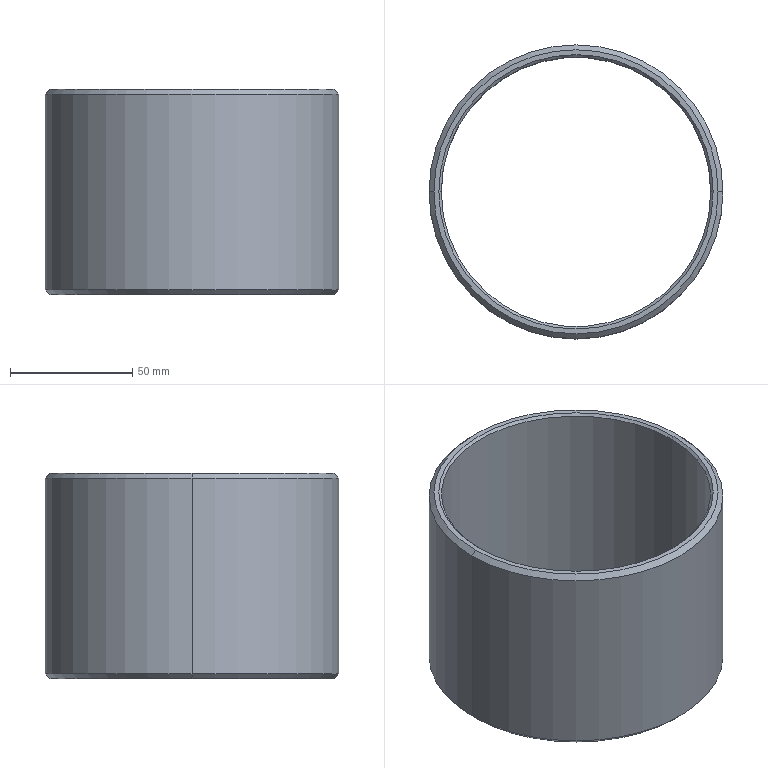Part | SolidWorks | features Chamfer 2, Extrusion 1 | 1 solid | 14 faces | box 120 x 120 x 84 mm | volume 149900 mm3 | cone 8 | cylinder 4 | plane 2 | commonest cylinder face diameters 110 x2 120 x2
STEP:
#1=CARTESIAN_POINT('',(-55.,0.,41.));
#2=VERTEX_POINT('',#1);
#3=CARTESIAN_POINT('',(55.,0.,41.));
#4=VERTEX_POINT('',#3);
#5=CARTESIAN_POINT('',(0.,0.,41.));
#6=DIRECTION('',(0.,0.,1.));
#7=DIRECTION('',(1.,0.,0.));
#8=AXIS2_PLACEMENT_3D('',#5,#6,#7);
#9=CIRCLE('',#8,55.);
#10=EDGE_CURVE('',#2,#4,#9,.T.);
#11=ORIENTED_EDGE('',*,*,#10,.F.);
#12=CARTESIAN_POINT('',(-56.,0.,42.));
#13=VERTEX_POINT('',#12);
#14=CARTESIAN_POINT('',(-55.,0.,41.));
#15=DIRECTION('',(-0.7071,0.,0.7071));
#16=VECTOR('',#15,1000.);
#17=LINE('',#14,#16);
#18=EDGE_CURVE('',#2,#13,#17,.T.);
#19=ORIENTED_EDGE('',*,*,#18,.T.);
#20=CARTESIAN_POINT('',(56.,0.,42.));
#21=VERTEX_POINT('',#20);
#22=CARTESIAN_POINT('',(0.,0.,42.));
#23=DIRECTION('',(0.,0.,-1.));
#24=DIRECTION('',(1.,0.,0.));
#25=AXIS2_PLACEMENT_3D('',#22,#23,#24);
#26=CIRCLE('',#25,56.);
#27=EDGE_CURVE('',#21,#13,#26,.T.);
#28=ORIENTED_EDGE('',*,*,#27,.F.);
#29=CARTESIAN_POINT('',(55.,0.,41.));
#30=DIRECTION('',(0.7071,0.,0.7071));
#31=VECTOR('',#30,1000.);
#32=LINE('',#29,#31);
#33=EDGE_CURVE('',#4,#21,#32,.T.);
#34=ORIENTED_EDGE('',*,*,#33,.F.);
#35=EDGE_LOOP('',(#11,#19,#28,#34));
#36=FACE_OUTER_BOUND('',#35,.T.);
#37=CARTESIAN_POINT('',(0.,0.,41.));
#38=DIRECTION('',(0.,0.,1.));
#39=DIRECTION('',(1.,0.,0.));
#40=AXIS2_PLACEMENT_3D('',#37,#38,#39);
#41=CONICAL_SURFACE('',#40,55.,0.7854);
#42=ADVANCED_FACE('',(#36),#41,.F.);
#43=CARTESIAN_POINT('',(55.,0.,-41.));
#44=VERTEX_POINT('',#43);
#45=CARTESIAN_POINT('',(-55.,0.,-41.));
#46=VERTEX_POINT('',#45);
#47=CARTESIAN_POINT('',(0.,0.,-41.));
#48=DIRECTION('',(0.,0.,-1.));
#49=DIRECTION('',(1.,0.,0.));
#50=AXIS2_PLACEMENT_3D('',#47,#48,#49);
#51=CIRCLE('',#50,55.);
#52=EDGE_CURVE('',#44,#46,#51,.T.);
#53=ORIENTED_EDGE('',*,*,#52,.F.);
#54=CARTESIAN_POINT('',(56.,0.,-42.));
#55=VERTEX_POINT('',#54);
#56=CARTESIAN_POINT('',(56.,0.,-42.));
#57=DIRECTION('',(0.7071,0.,-0.7071));
#58=VECTOR('',#57,1000.);
#59=LINE('',#56,#58);
#60=EDGE_CURVE('',#44,#55,#59,.T.);
#61=ORIENTED_EDGE('',*,*,#60,.T.);
#62=CARTESIAN_POINT('',(-56.,0.,-42.));
#63=VERTEX_POINT('',#62);
#64=CARTESIAN_POINT('',(0.,0.,-42.));
#65=DIRECTION('',(0.,0.,1.));
#66=DIRECTION('',(1.,0.,0.));
#67=AXIS2_PLACEMENT_3D('',#64,#65,#66);
#68=CIRCLE('',#67,56.);
#69=EDGE_CURVE('',#63,#55,#68,.T.);
#70=ORIENTED_EDGE('',*,*,#69,.F.);
#71=CARTESIAN_POINT('',(-56.,0.,-42.));
#72=DIRECTION('',(-0.7071,0.,-0.7071));
#73=VECTOR('',#72,1000.);
#74=LINE('',#71,#73);
#75=EDGE_CURVE('',#46,#63,#74,.T.);
#76=ORIENTED_EDGE('',*,*,#75,.F.);
#77=EDGE_LOOP('',(#53,#61,#70,#76));
#78=FACE_OUTER_BOUND('',#77,.T.);
#79=CARTESIAN_POINT('',(0.,0.,-42.));
#80=DIRECTION('',(0.,0.,-1.));
#81=DIRECTION('',(-1.,0.,0.));
#82=AXIS2_PLACEMENT_3D('',#79,#80,#81);
#83=CONICAL_SURFACE('',#82,56.,0.7854);
#84=ADVANCED_FACE('',(#78),#83,.F.);
#85=CARTESIAN_POINT('',(-58.,0.,-42.));
#86=VERTEX_POINT('',#85);
#87=CARTESIAN_POINT('',(58.,0.,-42.));
#88=VERTEX_POINT('',#87);
#89=CARTESIAN_POINT('',(0.,0.,-42.));
#90=DIRECTION('',(0.,0.,-1.));
#91=DIRECTION('',(1.,0.,0.));
#92=AXIS2_PLACEMENT_3D('',#89,#90,#91);
#93=CIRCLE('',#92,58.);
#94=EDGE_CURVE('',#86,#88,#93,.T.);
#95=ORIENTED_EDGE('',*,*,#94,.F.);
#96=CARTESIAN_POINT('',(-60.,0.,-40.));
#97=VERTEX_POINT('',#96);
#98=CARTESIAN_POINT('',(-60.,0.,-40.));
#99=DIRECTION('',(-0.7071,0.,0.7071));
#100=VECTOR('',#99,1000.);
#101=LINE('',#98,#100);
#102=EDGE_CURVE('',#86,#97,#101,.T.);
#103=ORIENTED_EDGE('',*,*,#102,.T.);
#104=CARTESIAN_POINT('',(60.,0.,-40.));
#105=VERTEX_POINT('',#104);
#106=CARTESIAN_POINT('',(0.,0.,-40.));
#107=DIRECTION('',(0.,0.,1.));
#108=DIRECTION('',(1.,0.,0.));
#109=AXIS2_PLACEMENT_3D('',#106,#107,#108);
#110=CIRCLE('',#109,60.);
#111=EDGE_CURVE('',#105,#97,#110,.T.);
#112=ORIENTED_EDGE('',*,*,#111,.F.);
#113=CARTESIAN_POINT('',(60.,0.,-40.));
#114=DIRECTION('',(0.7071,0.,0.7071));
#115=VECTOR('',#114,1000.);
#116=LINE('',#113,#115);
#117=EDGE_CURVE('',#88,#105,#116,.T.);
#118=ORIENTED_EDGE('',*,*,#117,.F.);
#119=EDGE_LOOP('',(#95,#103,#112,#118));
#120=FACE_OUTER_BOUND('',#119,.T.);
#121=CARTESIAN_POINT('',(0.,0.,-40.));
#122=DIRECTION('',(0.,0.,1.));
#123=DIRECTION('',(1.,0.,0.));
#124=AXIS2_PLACEMENT_3D('',#121,#122,#123);
#125=CONICAL_SURFACE('',#124,60.,0.7854);
#126=ADVANCED_FACE('',(#120),#125,.T.);
#127=CARTESIAN_POINT('',(58.,0.,42.));
#128=VERTEX_POINT('',#127);
#129=CARTESIAN_POINT('',(-58.,0.,42.));
#130=VERTEX_POINT('',#129);
#131=CARTESIAN_POINT('',(0.,0.,42.));
#132=DIRECTION('',(0.,0.,1.));
#133=DIRECTION('',(1.,0.,0.));
#134=AXIS2_PLACEMENT_3D('',#131,#132,#133);
#135=CIRCLE('',#134,58.);
#136=EDGE_CURVE('',#128,#130,#135,.T.);
#137=ORIENTED_EDGE('',*,*,#136,.F.);
#138=CARTESIAN_POINT('',(60.,0.,40.));
#139=VERTEX_POINT('',#138);
#140=CARTESIAN_POINT('',(58.,0.,42.));
#141=DIRECTION('',(0.7071,0.,-0.7071));
#142=VECTOR('',#141,1000.);
#143=LINE('',#140,#142);
#144=EDGE_CURVE('',#128,#139,#143,.T.);
#145=ORIENTED_EDGE('',*,*,#144,.T.);
#146=CARTESIAN_POINT('',(-60.,0.,40.));
#147=VERTEX_POINT('',#146);
#148=CARTESIAN_POINT('',(0.,0.,40.));
#149=DIRECTION('',(0.,0.,-1.));
#150=DIRECTION('',(1.,0.,0.));
#151=AXIS2_PLACEMENT_3D('',#148,#149,#150);
#152=CIRCLE('',#151,60.);
#153=EDGE_CURVE('',#147,#139,#152,.T.);
#154=ORIENTED_EDGE('',*,*,#153,.F.);
#155=CARTESIAN_POINT('',(-58.,0.,42.));
#156=DIRECTION('',(-0.7071,0.,-0.7071));
#157=VECTOR('',#156,1000.);
#158=LINE('',#155,#157);
#159=EDGE_CURVE('',#130,#147,#158,.T.);
#160=ORIENTED_EDGE('',*,*,#159,.F.);
#161=EDGE_LOOP('',(#137,#145,#154,#160));
#162=FACE_OUTER_BOUND('',#161,.T.);
#163=CARTESIAN_POINT('',(0.,0.,42.));
#164=DIRECTION('',(0.,0.,-1.));
#165=DIRECTION('',(-1.,0.,0.));
#166=AXIS2_PLACEMENT_3D('',#163,#164,#165);
#167=CONICAL_SURFACE('',#166,58.,0.7854);
#168=ADVANCED_FACE('',(#162),#167,.T.);
#169=ORIENTED_EDGE('',*,*,#10,.T.);
#170=CARTESIAN_POINT('',(55.,0.,42.));
#171=DIRECTION('',(0.,0.,-1.));
#172=VECTOR('',#171,1000.);
#173=LINE('',#170,#172);
#174=EDGE_CURVE('',#4,#44,#173,.T.);
#175=ORIENTED_EDGE('',*,*,#174,.T.);
#176=ORIENTED_EDGE('',*,*,#52,.T.);
#177=CARTESIAN_POINT('',(-55.,0.,42.));
#178=DIRECTION('',(0.,0.,-1.));
#179=VECTOR('',#178,1000.);
#180=LINE('',#177,#179);
#181=EDGE_CURVE('',#2,#46,#180,.T.);
#182=ORIENTED_EDGE('',*,*,#181,.F.);
#183=EDGE_LOOP('',(#169,#175,#176,#182));
#184=FACE_OUTER_BOUND('',#183,.T.);
#185=CARTESIAN_POINT('',(0.,0.,42.));
#186=DIRECTION('',(0.,0.,-1.));
#187=DIRECTION('',(-1.,0.,0.));
#188=AXIS2_PLACEMENT_3D('',#185,#186,#187);
#189=CYLINDRICAL_SURFACE('',#188,55.);
#190=ADVANCED_FACE('',(#184),#189,.F.);
#191=ORIENTED_EDGE('',*,*,#153,.T.);
#192=CARTESIAN_POINT('',(60.,0.,42.));
#193=DIRECTION('',(0.,0.,-1.));
#194=VECTOR('',#193,1000.);
#195=LINE('',#192,#194);
#196=EDGE_CURVE('',#139,#105,#195,.T.);
#197=ORIENTED_EDGE('',*,*,#196,.T.);
#198=ORIENTED_EDGE('',*,*,#111,.T.);
#199=CARTESIAN_POINT('',(-60.,0.,42.));
#200=DIRECTION('',(0.,0.,-1.));
#201=VECTOR('',#200,1000.);
#202=LINE('',#199,#201);
#203=EDGE_CURVE('',#147,#97,#202,.T.);
#204=ORIENTED_EDGE('',*,*,#203,.F.);
#205=EDGE_LOOP('',(#191,#197,#198,#204));
#206=FACE_OUTER_BOUND('',#205,.T.);
#207=CARTESIAN_POINT('',(0.,0.,42.));
#208=DIRECTION('',(0.,0.,-1.));
#209=DIRECTION('',(-1.,0.,0.));
#210=AXIS2_PLACEMENT_3D('',#207,#208,#209);
#211=CYLINDRICAL_SURFACE('',#210,60.);
#212=ADVANCED_FACE('',(#206),#211,.T.);
#213=ORIENTED_EDGE('',*,*,#27,.T.);
#214=CARTESIAN_POINT('',(0.,0.,42.));
#215=DIRECTION('',(0.,0.,-1.));
#216=DIRECTION('',(1.,0.,0.));
#217=AXIS2_PLACEMENT_3D('',#214,#215,#216);
#218=CIRCLE('',#217,56.);
#219=EDGE_CURVE('',#13,#21,#218,.T.);
#220=ORIENTED_EDGE('',*,*,#219,.T.);
#221=EDGE_LOOP('',(#213,#220));
#222=FACE_BOUND('',#221,.T.);
#223=CARTESIAN_POINT('',(0.,0.,42.));
#224=DIRECTION('',(0.,0.,1.));
#225=DIRECTION('',(1.,0.,0.));
#226=AXIS2_PLACEMENT_3D('',#223,#224,#225);
#227=CIRCLE('',#226,58.);
#228=EDGE_CURVE('',#130,#128,#227,.T.);
#229=ORIENTED_EDGE('',*,*,#228,.T.);
#230=ORIENTED_EDGE('',*,*,#136,.T.);
#231=EDGE_LOOP('',(#229,#230));
#232=FACE_OUTER_BOUND('',#231,.T.);
#233=CARTESIAN_POINT('',(0.,0.,42.));
#234=DIRECTION('',(0.,0.,1.));
#235=DIRECTION('',(1.,0.,0.));
#236=AXIS2_PLACEMENT_3D('',#233,#234,#235);
#237=PLANE('',#236);
#238=ADVANCED_FACE('',(#222,#232),#237,.T.);
#239=ORIENTED_EDGE('',*,*,#69,.T.);
#240=CARTESIAN_POINT('',(0.,0.,-42.));
#241=DIRECTION('',(0.,0.,1.));
#242=DIRECTION('',(1.,0.,0.));
#243=AXIS2_PLACEMENT_3D('',#240,#241,#242);
#244=CIRCLE('',#243,56.);
#245=EDGE_CURVE('',#55,#63,#244,.T.);
#246=ORIENTED_EDGE('',*,*,#245,.T.);
#247=EDGE_LOOP('',(#239,#246));
#248=FACE_BOUND('',#247,.T.);
#249=CARTESIAN_POINT('',(0.,0.,-42.));
#250=DIRECTION('',(0.,0.,-1.));
#251=DIRECTION('',(1.,0.,0.));
#252=AXIS2_PLACEMENT_3D('',#249,#250,#251);
#253=CIRCLE('',#252,58.);
#254=EDGE_CURVE('',#88,#86,#253,.T.);
#255=ORIENTED_EDGE('',*,*,#254,.T.);
#256=ORIENTED_EDGE('',*,*,#94,.T.);
#257=EDGE_LOOP('',(#255,#256));
#258=FACE_OUTER_BOUND('',#257,.T.);
#259=CARTESIAN_POINT('',(0.,0.,-42.));
#260=DIRECTION('',(0.,0.,1.));
#261=DIRECTION('',(1.,0.,0.));
#262=AXIS2_PLACEMENT_3D('',#259,#260,#261);
#263=PLANE('',#262);
#264=ADVANCED_FACE('',(#248,#258),#263,.F.);
#265=ORIENTED_EDGE('',*,*,#196,.F.);
#266=CARTESIAN_POINT('',(0.,0.,40.));
#267=DIRECTION('',(0.,0.,-1.));
#268=DIRECTION('',(1.,0.,0.));
#269=AXIS2_PLACEMENT_3D('',#266,#267,#268);
#270=CIRCLE('',#269,60.);
#271=EDGE_CURVE('',#139,#147,#270,.T.);
#272=ORIENTED_EDGE('',*,*,#271,.T.);
#273=ORIENTED_EDGE('',*,*,#203,.T.);
#274=CARTESIAN_POINT('',(0.,0.,-40.));
#275=DIRECTION('',(0.,0.,1.));
#276=DIRECTION('',(1.,0.,0.));
#277=AXIS2_PLACEMENT_3D('',#274,#275,#276);
#278=CIRCLE('',#277,60.);
#279=EDGE_CURVE('',#97,#105,#278,.T.);
#280=ORIENTED_EDGE('',*,*,#279,.T.);
#281=EDGE_LOOP('',(#265,#272,#273,#280));
#282=FACE_OUTER_BOUND('',#281,.T.);
#283=CARTESIAN_POINT('',(0.,0.,42.));
#284=DIRECTION('',(0.,0.,-1.));
#285=DIRECTION('',(-1.,0.,0.));
#286=AXIS2_PLACEMENT_3D('',#283,#284,#285);
#287=CYLINDRICAL_SURFACE('',#286,60.);
#288=ADVANCED_FACE('',(#282),#287,.T.);
#289=ORIENTED_EDGE('',*,*,#174,.F.);
#290=CARTESIAN_POINT('',(0.,0.,41.));
#291=DIRECTION('',(0.,0.,1.));
#292=DIRECTION('',(1.,0.,0.));
#293=AXIS2_PLACEMENT_3D('',#290,#291,#292);
#294=CIRCLE('',#293,55.);
#295=EDGE_CURVE('',#4,#2,#294,.T.);
#296=ORIENTED_EDGE('',*,*,#295,.T.);
#297=ORIENTED_EDGE('',*,*,#181,.T.);
#298=CARTESIAN_POINT('',(0.,0.,-41.));
#299=DIRECTION('',(0.,0.,-1.));
#300=DIRECTION('',(1.,0.,0.));
#301=AXIS2_PLACEMENT_3D('',#298,#299,#300);
#302=CIRCLE('',#301,55.);
#303=EDGE_CURVE('',#46,#44,#302,.T.);
#304=ORIENTED_EDGE('',*,*,#303,.T.);
#305=EDGE_LOOP('',(#289,#296,#297,#304));
#306=FACE_OUTER_BOUND('',#305,.T.);
#307=CARTESIAN_POINT('',(0.,0.,42.));
#308=DIRECTION('',(0.,0.,-1.));
#309=DIRECTION('',(-1.,0.,0.));
#310=AXIS2_PLACEMENT_3D('',#307,#308,#309);
#311=CYLINDRICAL_SURFACE('',#310,55.);
#312=ADVANCED_FACE('',(#306),#311,.F.);
#313=ORIENTED_EDGE('',*,*,#144,.F.);
#314=ORIENTED_EDGE('',*,*,#228,.F.);
#315=ORIENTED_EDGE('',*,*,#159,.T.);
#316=ORIENTED_EDGE('',*,*,#271,.F.);
#317=EDGE_LOOP('',(#313,#314,#315,#316));
#318=FACE_OUTER_BOUND('',#317,.T.);
#319=CARTESIAN_POINT('',(0.,0.,42.));
#320=DIRECTION('',(0.,0.,-1.));
#321=DIRECTION('',(-1.,0.,0.));
#322=AXIS2_PLACEMENT_3D('',#319,#320,#321);
#323=CONICAL_SURFACE('',#322,58.,0.7854);
#324=ADVANCED_FACE('',(#318),#323,.T.);
#325=ORIENTED_EDGE('',*,*,#102,.F.);
#326=ORIENTED_EDGE('',*,*,#254,.F.);
#327=ORIENTED_EDGE('',*,*,#117,.T.);
#328=ORIENTED_EDGE('',*,*,#279,.F.);
#329=EDGE_LOOP('',(#325,#326,#327,#328));
#330=FACE_OUTER_BOUND('',#329,.T.);
#331=CARTESIAN_POINT('',(0.,0.,-40.));
#332=DIRECTION('',(0.,0.,1.));
#333=DIRECTION('',(1.,0.,0.));
#334=AXIS2_PLACEMENT_3D('',#331,#332,#333);
#335=CONICAL_SURFACE('',#334,60.,0.7854);
#336=ADVANCED_FACE('',(#330),#335,.T.);
#337=ORIENTED_EDGE('',*,*,#60,.F.);
#338=ORIENTED_EDGE('',*,*,#303,.F.);
#339=ORIENTED_EDGE('',*,*,#75,.T.);
#340=ORIENTED_EDGE('',*,*,#245,.F.);
#341=EDGE_LOOP('',(#337,#338,#339,#340));
#342=FACE_OUTER_BOUND('',#341,.T.);
#343=CARTESIAN_POINT('',(0.,0.,-42.));
#344=DIRECTION('',(0.,0.,-1.));
#345=DIRECTION('',(-1.,0.,0.));
#346=AXIS2_PLACEMENT_3D('',#343,#344,#345);
#347=CONICAL_SURFACE('',#346,56.,0.7854);
#348=ADVANCED_FACE('',(#342),#347,.F.);
#349=ORIENTED_EDGE('',*,*,#18,.F.);
#350=ORIENTED_EDGE('',*,*,#295,.F.);
#351=ORIENTED_EDGE('',*,*,#33,.T.);
#352=ORIENTED_EDGE('',*,*,#219,.F.);
#353=EDGE_LOOP('',(#349,#350,#351,#352));
#354=FACE_OUTER_BOUND('',#353,.T.);
#355=CARTESIAN_POINT('',(0.,0.,41.));
#356=DIRECTION('',(0.,0.,1.));
#357=DIRECTION('',(1.,0.,0.));
#358=AXIS2_PLACEMENT_3D('',#355,#356,#357);
#359=CONICAL_SURFACE('',#358,55.,0.7854);
#360=ADVANCED_FACE('',(#354),#359,.F.);
#361=CLOSED_SHELL('',(#42,#84,#126,#168,#190,#212,#238,#264,#288,#312,#324,#336,#348,#360));
#362=MANIFOLD_SOLID_BREP('',#361);
#363=CARTESIAN_POINT('',(0.,0.,0.));
#364=DIRECTION('',(0.,0.,1.));
#365=DIRECTION('',(1.,0.,0.));
#366=AXIS2_PLACEMENT_3D('',#363,#364,#365);
#367=(LENGTH_UNIT()NAMED_UNIT(*)SI_UNIT(.MILLI.,.METRE.));
#368=UNCERTAINTY_MEASURE_WITH_UNIT(LENGTH_MEASURE(0.00001),#367,'','');
#369=(NAMED_UNIT(*)PLANE_ANGLE_UNIT()SI_UNIT($,.RADIAN.));
#370=(NAMED_UNIT(*)SI_UNIT($,.STERADIAN.)SOLID_ANGLE_UNIT());
#371=(GEOMETRIC_REPRESENTATION_CONTEXT(3)GLOBAL_UNCERTAINTY_ASSIGNED_CONTEXT((#368))GLOBAL_UNIT_ASSIGNED_CONTEXT((#367,#369,#370))REPRESENTATION_CONTEXT('',''));
#372=ADVANCED_BREP_SHAPE_REPRESENTATION('',(#362,#366),#371);